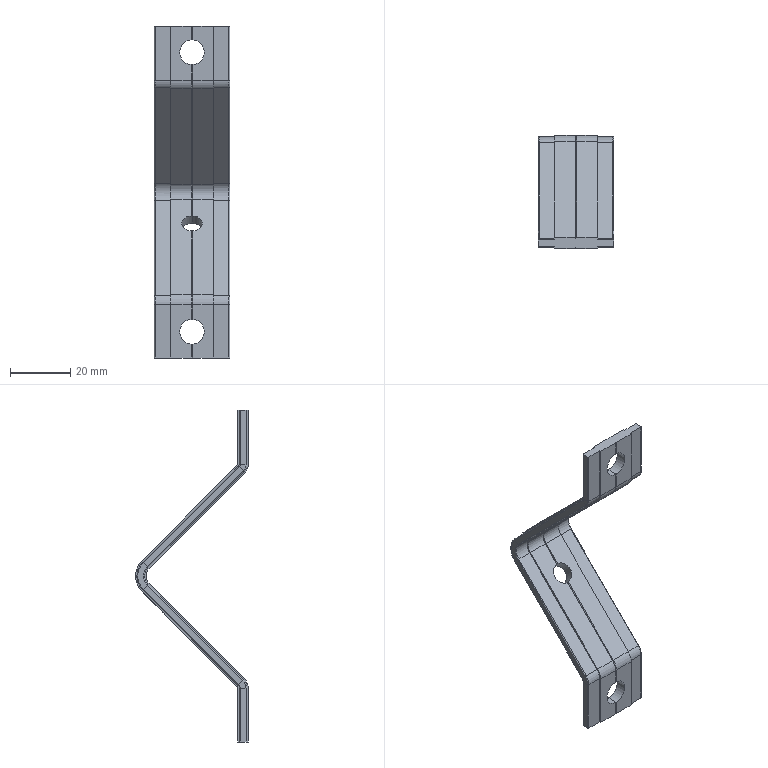Part | STEP file | PN_0026_Default<As Machined> | 1 solid | 174 faces | box 25 x 37.475 x 110 mm | volume 10034 mm3 | plane 104 | cylinder 46 | cone 12 | torus 12 | commonest cylinder face diameters 0.6 x16 7 x4 8.2 x4 0.5 x2 1.5 x2 2.5 x2